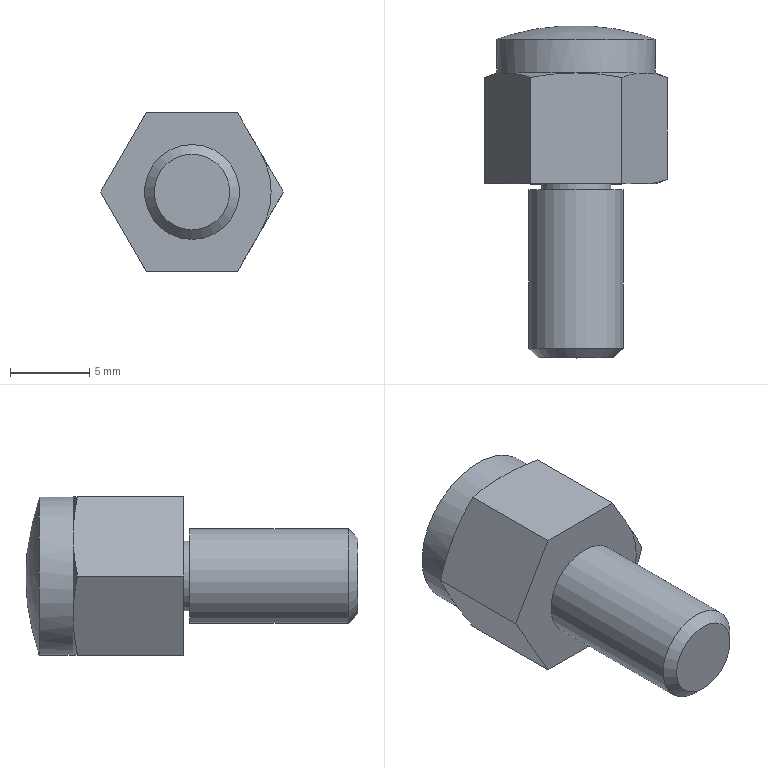Part | NX | features BREP 1 | 1 solid | 21 faces | box 11.547 x 21 x 10 mm | volume 1111 mm3 | plane 9 | cone 8 | cylinder 3 | sphere 1 | commonest cylinder face diameters 4.4 x1 6 x1 10 x1
STEP:
#1=CARTESIAN_POINT('',(4.33,0.5,-2.5));
#2=VERTEX_POINT('',#1);
#3=CARTESIAN_POINT('',(4.33,0.5,2.5));
#4=VERTEX_POINT('',#3);
#5=CARTESIAN_POINT('',(0.,0.5,0.));
#6=DIRECTION('',(0.,-1.,0.));
#7=DIRECTION('',(0.,0.,-1.));
#8=AXIS2_PLACEMENT_3D('',#5,#6,#7);
#9=CIRCLE('',#8,5.);
#10=EDGE_CURVE('',#2,#4,#9,.T.);
#11=ORIENTED_EDGE('',*,*,#10,.F.);
#12=CARTESIAN_POINT('',(5.774,0.7815,0.));
#13=VERTEX_POINT('',#12);
#14=CARTESIAN_POINT('',(4.33,0.5,-2.5));
#15=CARTESIAN_POINT('',(4.816,0.5,-1.659));
#16=CARTESIAN_POINT('',(5.296,0.6078,-0.8266));
#17=CARTESIAN_POINT('',(5.774,0.7815,0.));
#18=B_SPLINE_CURVE_WITH_KNOTS('',3,(#14,#15,#16,#17),.UNSPECIFIED.,.F.,.F.,(4,4),(0.,0.0029),.UNSPECIFIED.);
#19=EDGE_CURVE('',#2,#13,#18,.T.);
#20=ORIENTED_EDGE('',*,*,#19,.T.);
#21=CARTESIAN_POINT('',(5.774,0.7815,0.));
#22=CARTESIAN_POINT('',(5.296,0.6078,0.8266));
#23=CARTESIAN_POINT('',(4.816,0.5,1.659));
#24=CARTESIAN_POINT('',(4.33,0.5,2.5));
#25=B_SPLINE_CURVE_WITH_KNOTS('',3,(#21,#22,#23,#24),.UNSPECIFIED.,.F.,.F.,(4,4),(0.,0.0029),.UNSPECIFIED.);
#26=EDGE_CURVE('',#13,#4,#25,.T.);
#27=ORIENTED_EDGE('',*,*,#26,.T.);
#28=EDGE_LOOP('',(#11,#20,#27));
#29=FACE_BOUND('',#28,.T.);
#30=CARTESIAN_POINT('',(0.,4.,0.));
#31=DIRECTION('',(0.,1.,0.));
#32=DIRECTION('',(0.,0.,-1.));
#33=AXIS2_PLACEMENT_3D('',#30,#31,#32);
#34=CONICAL_SURFACE('',#33,14.616,1.222);
#35=ADVANCED_FACE('',(#29),#34,.T.);
#36=CARTESIAN_POINT('',(0.,0.5,-2.2));
#37=VERTEX_POINT('',#36);
#38=CARTESIAN_POINT('',(0.,0.5,0.));
#39=DIRECTION('',(0.,-1.,0.));
#40=DIRECTION('',(0.,0.,-1.));
#41=AXIS2_PLACEMENT_3D('',#38,#39,#40);
#42=CIRCLE('',#41,2.2);
#43=EDGE_CURVE('',#37,#37,#42,.T.);
#44=ORIENTED_EDGE('',*,*,#43,.F.);
#45=EDGE_LOOP('',(#44));
#46=FACE_BOUND('',#45,.T.);
#47=CARTESIAN_POINT('',(2.887,0.5,-5.));
#48=VERTEX_POINT('',#47);
#49=CARTESIAN_POINT('',(-2.887,0.5,-5.));
#50=VERTEX_POINT('',#49);
#51=CARTESIAN_POINT('',(5.,0.5,-5.));
#52=DIRECTION('',(-1.,0.,0.));
#53=VECTOR('',#52,1000.);
#54=LINE('',#51,#53);
#55=EDGE_CURVE('',#48,#50,#54,.T.);
#56=ORIENTED_EDGE('',*,*,#55,.F.);
#57=CARTESIAN_POINT('',(5.58,0.5,-0.3349));
#58=DIRECTION('',(-0.5,0.,-0.866));
#59=VECTOR('',#58,1000.);
#60=LINE('',#57,#59);
#61=EDGE_CURVE('',#2,#48,#60,.T.);
#62=ORIENTED_EDGE('',*,*,#61,.F.);
#63=ORIENTED_EDGE('',*,*,#10,.T.);
#64=CARTESIAN_POINT('',(2.887,0.5,5.));
#65=VERTEX_POINT('',#64);
#66=CARTESIAN_POINT('',(2.887,0.5,5.));
#67=DIRECTION('',(-0.5,0.,0.866));
#68=VECTOR('',#67,1000.);
#69=LINE('',#66,#68);
#70=EDGE_CURVE('',#4,#65,#69,.T.);
#71=ORIENTED_EDGE('',*,*,#70,.T.);
#72=CARTESIAN_POINT('',(-2.887,0.5,5.));
#73=VERTEX_POINT('',#72);
#74=CARTESIAN_POINT('',(-2.887,0.5,5.));
#75=DIRECTION('',(-1.,0.,0.));
#76=VECTOR('',#75,1000.);
#77=LINE('',#74,#76);
#78=EDGE_CURVE('',#65,#73,#77,.T.);
#79=ORIENTED_EDGE('',*,*,#78,.T.);
#80=CARTESIAN_POINT('',(-5.774,0.5,0.));
#81=VERTEX_POINT('',#80);
#82=CARTESIAN_POINT('',(-5.774,0.5,0.));
#83=DIRECTION('',(-0.5,0.,-0.866));
#84=VECTOR('',#83,1000.);
#85=LINE('',#82,#84);
#86=EDGE_CURVE('',#73,#81,#85,.T.);
#87=ORIENTED_EDGE('',*,*,#86,.T.);
#88=CARTESIAN_POINT('',(-3.08,0.5,-4.665));
#89=DIRECTION('',(-0.5,0.,0.866));
#90=VECTOR('',#89,1000.);
#91=LINE('',#88,#90);
#92=EDGE_CURVE('',#50,#81,#91,.T.);
#93=ORIENTED_EDGE('',*,*,#92,.F.);
#94=EDGE_LOOP('',(#56,#62,#63,#71,#79,#87,#93));
#95=FACE_BOUND('',#94,.T.);
#96=CARTESIAN_POINT('',(5.,0.5,0.));
#97=DIRECTION('',(0.,1.,0.));
#98=DIRECTION('',(0.,0.,-1.));
#99=AXIS2_PLACEMENT_3D('',#96,#97,#98);
#100=PLANE('',#99);
#101=ADVANCED_FACE('',(#46,#95),#100,.F.);
#102=CARTESIAN_POINT('',(-2.887,7.218,-5.));
#103=VERTEX_POINT('',#102);
#104=CARTESIAN_POINT('',(-2.887,15.,-5.));
#105=DIRECTION('',(0.,-1.,0.));
#106=VECTOR('',#105,1000.);
#107=LINE('',#104,#106);
#108=EDGE_CURVE('',#103,#50,#107,.T.);
#109=ORIENTED_EDGE('',*,*,#108,.T.);
#110=ORIENTED_EDGE('',*,*,#92,.T.);
#111=CARTESIAN_POINT('',(-5.774,7.218,0.));
#112=VERTEX_POINT('',#111);
#113=CARTESIAN_POINT('',(-5.774,15.,0.));
#114=DIRECTION('',(0.,-1.,0.));
#115=VECTOR('',#114,1000.);
#116=LINE('',#113,#115);
#117=EDGE_CURVE('',#112,#81,#116,.T.);
#118=ORIENTED_EDGE('',*,*,#117,.F.);
#119=CARTESIAN_POINT('',(-4.33,7.5,-2.5));
#120=VERTEX_POINT('',#119);
#121=CARTESIAN_POINT('',(-4.33,7.5,-2.5));
#122=CARTESIAN_POINT('',(-4.816,7.5,-1.659));
#123=CARTESIAN_POINT('',(-5.296,7.392,-0.8266));
#124=CARTESIAN_POINT('',(-5.774,7.218,0.));
#125=B_SPLINE_CURVE_WITH_KNOTS('',3,(#121,#122,#123,#124),.UNSPECIFIED.,.F.,.F.,(4,4),(0.,0.0029),.UNSPECIFIED.);
#126=EDGE_CURVE('',#120,#112,#125,.T.);
#127=ORIENTED_EDGE('',*,*,#126,.F.);
#128=CARTESIAN_POINT('',(-2.887,7.218,-5.));
#129=CARTESIAN_POINT('',(-3.364,7.392,-4.173));
#130=CARTESIAN_POINT('',(-3.844,7.5,-3.341));
#131=CARTESIAN_POINT('',(-4.33,7.5,-2.5));
#132=B_SPLINE_CURVE_WITH_KNOTS('',3,(#128,#129,#130,#131),.UNSPECIFIED.,.F.,.F.,(4,4),(0.,0.0029),.UNSPECIFIED.);
#133=EDGE_CURVE('',#103,#120,#132,.T.);
#134=ORIENTED_EDGE('',*,*,#133,.F.);
#135=EDGE_LOOP('',(#109,#110,#118,#127,#134));
#136=FACE_BOUND('',#135,.T.);
#137=CARTESIAN_POINT('',(-2.887,15.,-5.));
#138=DIRECTION('',(0.866,0.,0.5));
#139=DIRECTION('',(-0.5,0.,0.866));
#140=AXIS2_PLACEMENT_3D('',#137,#138,#139);
#141=PLANE('',#140);
#142=ADVANCED_FACE('',(#136),#141,.F.);
#143=CARTESIAN_POINT('',(2.887,7.218,-5.));
#144=VERTEX_POINT('',#143);
#145=CARTESIAN_POINT('',(2.887,15.,-5.));
#146=DIRECTION('',(0.,-1.,0.));
#147=VECTOR('',#146,1000.);
#148=LINE('',#145,#147);
#149=EDGE_CURVE('',#144,#48,#148,.T.);
#150=ORIENTED_EDGE('',*,*,#149,.T.);
#151=ORIENTED_EDGE('',*,*,#55,.T.);
#152=ORIENTED_EDGE('',*,*,#108,.F.);
#153=CARTESIAN_POINT('',(0.,7.5,-5.));
#154=VERTEX_POINT('',#153);
#155=CARTESIAN_POINT('',(0.,7.5,-5.));
#156=CARTESIAN_POINT('',(-0.9714,7.5,-5.));
#157=CARTESIAN_POINT('',(-1.932,7.392,-5.));
#158=CARTESIAN_POINT('',(-2.887,7.218,-5.));
#159=B_SPLINE_CURVE_WITH_KNOTS('',3,(#155,#156,#157,#158),.UNSPECIFIED.,.F.,.F.,(4,4),(0.,0.0029),.UNSPECIFIED.);
#160=EDGE_CURVE('',#154,#103,#159,.T.);
#161=ORIENTED_EDGE('',*,*,#160,.F.);
#162=CARTESIAN_POINT('',(2.887,7.218,-5.));
#163=CARTESIAN_POINT('',(1.932,7.392,-5.));
#164=CARTESIAN_POINT('',(0.9714,7.5,-5.));
#165=CARTESIAN_POINT('',(0.,7.5,-5.));
#166=B_SPLINE_CURVE_WITH_KNOTS('',3,(#162,#163,#164,#165),.UNSPECIFIED.,.F.,.F.,(4,4),(0.,0.0029),.UNSPECIFIED.);
#167=EDGE_CURVE('',#144,#154,#166,.T.);
#168=ORIENTED_EDGE('',*,*,#167,.F.);
#169=EDGE_LOOP('',(#150,#151,#152,#161,#168));
#170=FACE_BOUND('',#169,.T.);
#171=CARTESIAN_POINT('',(2.887,15.,-5.));
#172=DIRECTION('',(0.,0.,1.));
#173=DIRECTION('',(-1.,0.,0.));
#174=AXIS2_PLACEMENT_3D('',#171,#172,#173);
#175=PLANE('',#174);
#176=ADVANCED_FACE('',(#170),#175,.F.);
#177=CARTESIAN_POINT('',(5.774,7.218,0.));
#178=VERTEX_POINT('',#177);
#179=CARTESIAN_POINT('',(5.774,15.,0.));
#180=DIRECTION('',(0.,-1.,0.));
#181=VECTOR('',#180,1000.);
#182=LINE('',#179,#181);
#183=EDGE_CURVE('',#178,#13,#182,.T.);
#184=ORIENTED_EDGE('',*,*,#183,.T.);
#185=ORIENTED_EDGE('',*,*,#19,.F.);
#186=ORIENTED_EDGE('',*,*,#61,.T.);
#187=ORIENTED_EDGE('',*,*,#149,.F.);
#188=CARTESIAN_POINT('',(4.33,7.5,-2.5));
#189=VERTEX_POINT('',#188);
#190=CARTESIAN_POINT('',(4.33,7.5,-2.5));
#191=CARTESIAN_POINT('',(3.844,7.5,-3.341));
#192=CARTESIAN_POINT('',(3.364,7.392,-4.173));
#193=CARTESIAN_POINT('',(2.887,7.218,-5.));
#194=B_SPLINE_CURVE_WITH_KNOTS('',3,(#190,#191,#192,#193),.UNSPECIFIED.,.F.,.F.,(4,4),(0.,0.0029),.UNSPECIFIED.);
#195=EDGE_CURVE('',#189,#144,#194,.T.);
#196=ORIENTED_EDGE('',*,*,#195,.F.);
#197=CARTESIAN_POINT('',(5.774,7.218,0.));
#198=CARTESIAN_POINT('',(5.296,7.392,-0.8266));
#199=CARTESIAN_POINT('',(4.816,7.5,-1.659));
#200=CARTESIAN_POINT('',(4.33,7.5,-2.5));
#201=B_SPLINE_CURVE_WITH_KNOTS('',3,(#197,#198,#199,#200),.UNSPECIFIED.,.F.,.F.,(4,4),(0.,0.0029),.UNSPECIFIED.);
#202=EDGE_CURVE('',#178,#189,#201,.T.);
#203=ORIENTED_EDGE('',*,*,#202,.F.);
#204=EDGE_LOOP('',(#184,#185,#186,#187,#196,#203));
#205=FACE_BOUND('',#204,.T.);
#206=CARTESIAN_POINT('',(5.774,15.,0.));
#207=DIRECTION('',(-0.866,0.,0.5));
#208=DIRECTION('',(-0.5,0.,-0.866));
#209=AXIS2_PLACEMENT_3D('',#206,#207,#208);
#210=PLANE('',#209);
#211=ADVANCED_FACE('',(#205),#210,.F.);
#212=CARTESIAN_POINT('',(2.887,7.218,5.));
#213=VERTEX_POINT('',#212);
#214=CARTESIAN_POINT('',(2.887,15.,5.));
#215=DIRECTION('',(0.,-1.,0.));
#216=VECTOR('',#215,1000.);
#217=LINE('',#214,#216);
#218=EDGE_CURVE('',#213,#65,#217,.T.);
#219=ORIENTED_EDGE('',*,*,#218,.T.);
#220=ORIENTED_EDGE('',*,*,#70,.F.);
#221=ORIENTED_EDGE('',*,*,#26,.F.);
#222=ORIENTED_EDGE('',*,*,#183,.F.);
#223=CARTESIAN_POINT('',(4.33,7.5,2.5));
#224=VERTEX_POINT('',#223);
#225=CARTESIAN_POINT('',(4.33,7.5,2.5));
#226=CARTESIAN_POINT('',(4.816,7.5,1.659));
#227=CARTESIAN_POINT('',(5.296,7.392,0.8266));
#228=CARTESIAN_POINT('',(5.774,7.218,0.));
#229=B_SPLINE_CURVE_WITH_KNOTS('',3,(#225,#226,#227,#228),.UNSPECIFIED.,.F.,.F.,(4,4),(0.,0.0029),.UNSPECIFIED.);
#230=EDGE_CURVE('',#224,#178,#229,.T.);
#231=ORIENTED_EDGE('',*,*,#230,.F.);
#232=CARTESIAN_POINT('',(2.887,7.218,5.));
#233=CARTESIAN_POINT('',(3.364,7.392,4.173));
#234=CARTESIAN_POINT('',(3.844,7.5,3.341));
#235=CARTESIAN_POINT('',(4.33,7.5,2.5));
#236=B_SPLINE_CURVE_WITH_KNOTS('',3,(#232,#233,#234,#235),.UNSPECIFIED.,.F.,.F.,(4,4),(0.,0.0029),.UNSPECIFIED.);
#237=EDGE_CURVE('',#213,#224,#236,.T.);
#238=ORIENTED_EDGE('',*,*,#237,.F.);
#239=EDGE_LOOP('',(#219,#220,#221,#222,#231,#238));
#240=FACE_BOUND('',#239,.T.);
#241=CARTESIAN_POINT('',(2.887,15.,5.));
#242=DIRECTION('',(-0.866,0.,-0.5));
#243=DIRECTION('',(0.5,0.,-0.866));
#244=AXIS2_PLACEMENT_3D('',#241,#242,#243);
#245=PLANE('',#244);
#246=ADVANCED_FACE('',(#240),#245,.F.);
#247=CARTESIAN_POINT('',(-2.887,7.218,5.));
#248=VERTEX_POINT('',#247);
#249=CARTESIAN_POINT('',(-2.887,15.,5.));
#250=DIRECTION('',(0.,-1.,0.));
#251=VECTOR('',#250,1000.);
#252=LINE('',#249,#251);
#253=EDGE_CURVE('',#248,#73,#252,.T.);
#254=ORIENTED_EDGE('',*,*,#253,.T.);
#255=ORIENTED_EDGE('',*,*,#78,.F.);
#256=ORIENTED_EDGE('',*,*,#218,.F.);
#257=CARTESIAN_POINT('',(0.,7.5,5.));
#258=VERTEX_POINT('',#257);
#259=CARTESIAN_POINT('',(0.,7.5,5.));
#260=CARTESIAN_POINT('',(0.9714,7.5,5.));
#261=CARTESIAN_POINT('',(1.932,7.392,5.));
#262=CARTESIAN_POINT('',(2.887,7.218,5.));
#263=B_SPLINE_CURVE_WITH_KNOTS('',3,(#259,#260,#261,#262),.UNSPECIFIED.,.F.,.F.,(4,4),(0.,0.0029),.UNSPECIFIED.);
#264=EDGE_CURVE('',#258,#213,#263,.T.);
#265=ORIENTED_EDGE('',*,*,#264,.F.);
#266=CARTESIAN_POINT('',(-2.887,7.218,5.));
#267=CARTESIAN_POINT('',(-1.932,7.392,5.));
#268=CARTESIAN_POINT('',(-0.9714,7.5,5.));
#269=CARTESIAN_POINT('',(0.,7.5,5.));
#270=B_SPLINE_CURVE_WITH_KNOTS('',3,(#266,#267,#268,#269),.UNSPECIFIED.,.F.,.F.,(4,4),(0.,0.0029),.UNSPECIFIED.);
#271=EDGE_CURVE('',#248,#258,#270,.T.);
#272=ORIENTED_EDGE('',*,*,#271,.F.);
#273=EDGE_LOOP('',(#254,#255,#256,#265,#272));
#274=FACE_BOUND('',#273,.T.);
#275=CARTESIAN_POINT('',(-2.887,15.,5.));
#276=DIRECTION('',(0.,0.,-1.));
#277=DIRECTION('',(1.,0.,0.));
#278=AXIS2_PLACEMENT_3D('',#275,#276,#277);
#279=PLANE('',#278);
#280=ADVANCED_FACE('',(#274),#279,.F.);
#281=ORIENTED_EDGE('',*,*,#117,.T.);
#282=ORIENTED_EDGE('',*,*,#86,.F.);
#283=ORIENTED_EDGE('',*,*,#253,.F.);
#284=CARTESIAN_POINT('',(-4.33,7.5,2.5));
#285=VERTEX_POINT('',#284);
#286=CARTESIAN_POINT('',(-4.33,7.5,2.5));
#287=CARTESIAN_POINT('',(-3.844,7.5,3.341));
#288=CARTESIAN_POINT('',(-3.364,7.392,4.173));
#289=CARTESIAN_POINT('',(-2.887,7.218,5.));
#290=B_SPLINE_CURVE_WITH_KNOTS('',3,(#286,#287,#288,#289),.UNSPECIFIED.,.F.,.F.,(4,4),(0.,0.0029),.UNSPECIFIED.);
#291=EDGE_CURVE('',#285,#248,#290,.T.);
#292=ORIENTED_EDGE('',*,*,#291,.F.);
#293=CARTESIAN_POINT('',(-5.774,7.218,0.));
#294=CARTESIAN_POINT('',(-5.296,7.392,0.8266));
#295=CARTESIAN_POINT('',(-4.816,7.5,1.659));
#296=CARTESIAN_POINT('',(-4.33,7.5,2.5));
#297=B_SPLINE_CURVE_WITH_KNOTS('',3,(#293,#294,#295,#296),.UNSPECIFIED.,.F.,.F.,(4,4),(0.,0.0029),.UNSPECIFIED.);
#298=EDGE_CURVE('',#112,#285,#297,.T.);
#299=ORIENTED_EDGE('',*,*,#298,.F.);
#300=EDGE_LOOP('',(#281,#282,#283,#292,#299));
#301=FACE_BOUND('',#300,.T.);
#302=CARTESIAN_POINT('',(-5.774,15.,0.));
#303=DIRECTION('',(0.866,0.,-0.5));
#304=DIRECTION('',(0.5,0.,0.866));
#305=AXIS2_PLACEMENT_3D('',#302,#303,#304);
#306=PLANE('',#305);
#307=ADVANCED_FACE('',(#301),#306,.F.);
#308=CARTESIAN_POINT('',(0.,9.642,-5.));
#309=VERTEX_POINT('',#308);
#310=CARTESIAN_POINT('',(0.,9.642,0.));
#311=DIRECTION('',(0.,-1.,0.));
#312=DIRECTION('',(0.,0.,-1.));
#313=AXIS2_PLACEMENT_3D('',#310,#311,#312);
#314=CIRCLE('',#313,5.);
#315=EDGE_CURVE('',#309,#309,#314,.T.);
#316=ORIENTED_EDGE('',*,*,#315,.F.);
#317=EDGE_LOOP('',(#316));
#318=FACE_BOUND('',#317,.T.);
#319=CARTESIAN_POINT('',(0.,-4.5,0.));
#320=DIRECTION('',(0.,0.,1.));
#321=DIRECTION('',(-1.,0.,0.));
#322=AXIS2_PLACEMENT_3D('',#319,#320,#321);
#323=SPHERICAL_SURFACE('',#322,15.);
#324=ADVANCED_FACE('',(#318),#323,.T.);
#325=CARTESIAN_POINT('',(0.,7.5,0.));
#326=DIRECTION('',(0.,-1.,0.));
#327=DIRECTION('',(0.,0.,-1.));
#328=AXIS2_PLACEMENT_3D('',#325,#326,#327);
#329=CIRCLE('',#328,5.);
#330=EDGE_CURVE('',#154,#189,#329,.T.);
#331=ORIENTED_EDGE('',*,*,#330,.T.);
#332=ORIENTED_EDGE('',*,*,#195,.T.);
#333=ORIENTED_EDGE('',*,*,#167,.T.);
#334=EDGE_LOOP('',(#331,#332,#333));
#335=FACE_BOUND('',#334,.T.);
#336=CARTESIAN_POINT('',(0.,7.5,0.));
#337=DIRECTION('',(0.,-1.,0.));
#338=DIRECTION('',(0.,0.,1.));
#339=AXIS2_PLACEMENT_3D('',#336,#337,#338);
#340=CONICAL_SURFACE('',#339,5.,1.222);
#341=ADVANCED_FACE('',(#335),#340,.T.);
#342=ORIENTED_EDGE('',*,*,#291,.T.);
#343=ORIENTED_EDGE('',*,*,#271,.T.);
#344=CARTESIAN_POINT('',(0.,7.5,0.));
#345=DIRECTION('',(0.,-1.,0.));
#346=DIRECTION('',(0.,0.,-1.));
#347=AXIS2_PLACEMENT_3D('',#344,#345,#346);
#348=CIRCLE('',#347,5.);
#349=EDGE_CURVE('',#258,#285,#348,.T.);
#350=ORIENTED_EDGE('',*,*,#349,.T.);
#351=EDGE_LOOP('',(#342,#343,#350));
#352=FACE_BOUND('',#351,.T.);
#353=CARTESIAN_POINT('',(0.,7.5,0.));
#354=DIRECTION('',(0.,-1.,0.));
#355=DIRECTION('',(0.,0.,1.));
#356=AXIS2_PLACEMENT_3D('',#353,#354,#355);
#357=CONICAL_SURFACE('',#356,5.,1.222);
#358=ADVANCED_FACE('',(#352),#357,.T.);
#359=CARTESIAN_POINT('',(0.,7.5,0.));
#360=DIRECTION('',(0.,-1.,0.));
#361=DIRECTION('',(0.,0.,-1.));
#362=AXIS2_PLACEMENT_3D('',#359,#360,#361);
#363=CIRCLE('',#362,5.);
#364=EDGE_CURVE('',#285,#120,#363,.T.);
#365=ORIENTED_EDGE('',*,*,#364,.T.);
#366=ORIENTED_EDGE('',*,*,#126,.T.);
#367=ORIENTED_EDGE('',*,*,#298,.T.);
#368=EDGE_LOOP('',(#365,#366,#367));
#369=FACE_BOUND('',#368,.T.);
#370=CARTESIAN_POINT('',(0.,7.5,0.));
#371=DIRECTION('',(0.,-1.,0.));
#372=DIRECTION('',(0.,0.,1.));
#373=AXIS2_PLACEMENT_3D('',#370,#371,#372);
#374=CONICAL_SURFACE('',#373,5.,1.222);
#375=ADVANCED_FACE('',(#369),#374,.T.);
#376=ORIENTED_EDGE('',*,*,#264,.T.);
#377=ORIENTED_EDGE('',*,*,#237,.T.);
#378=CARTESIAN_POINT('',(0.,7.5,0.));
#379=DIRECTION('',(0.,-1.,0.));
#380=DIRECTION('',(0.,0.,-1.));
#381=AXIS2_PLACEMENT_3D('',#378,#379,#380);
#382=CIRCLE('',#381,5.);
#383=EDGE_CURVE('',#224,#258,#382,.T.);
#384=ORIENTED_EDGE('',*,*,#383,.T.);
#385=EDGE_LOOP('',(#376,#377,#384));
#386=FACE_BOUND('',#385,.T.);
#387=CARTESIAN_POINT('',(0.,7.5,0.));
#388=DIRECTION('',(0.,-1.,0.));
#389=DIRECTION('',(0.,0.,1.));
#390=AXIS2_PLACEMENT_3D('',#387,#388,#389);
#391=CONICAL_SURFACE('',#390,5.,1.222);
#392=ADVANCED_FACE('',(#386),#391,.T.);
#393=CARTESIAN_POINT('',(0.,7.5,0.));
#394=DIRECTION('',(0.,-1.,0.));
#395=DIRECTION('',(0.,0.,-1.));
#396=AXIS2_PLACEMENT_3D('',#393,#394,#395);
#397=CIRCLE('',#396,5.);
#398=EDGE_CURVE('',#189,#224,#397,.T.);
#399=ORIENTED_EDGE('',*,*,#398,.F.);
#400=ORIENTED_EDGE('',*,*,#330,.F.);
#401=CARTESIAN_POINT('',(0.,7.5,0.));
#402=DIRECTION('',(0.,-1.,0.));
#403=DIRECTION('',(0.,0.,-1.));
#404=AXIS2_PLACEMENT_3D('',#401,#402,#403);
#405=CIRCLE('',#404,5.);
#406=EDGE_CURVE('',#120,#154,#405,.T.);
#407=ORIENTED_EDGE('',*,*,#406,.F.);
#408=ORIENTED_EDGE('',*,*,#364,.F.);
#409=ORIENTED_EDGE('',*,*,#349,.F.);
#410=ORIENTED_EDGE('',*,*,#383,.F.);
#411=EDGE_LOOP('',(#399,#400,#407,#408,#409,#410));
#412=FACE_BOUND('',#411,.T.);
#413=ORIENTED_EDGE('',*,*,#315,.T.);
#414=EDGE_LOOP('',(#413));
#415=FACE_BOUND('',#414,.T.);
#416=CARTESIAN_POINT('',(0.,-10.5,0.));
#417=DIRECTION('',(0.,-1.,0.));
#418=DIRECTION('',(0.,0.,1.));
#419=AXIS2_PLACEMENT_3D('',#416,#417,#418);
#420=CYLINDRICAL_SURFACE('',#419,5.);
#421=ADVANCED_FACE('',(#412,#415),#420,.T.);
#422=ORIENTED_EDGE('',*,*,#398,.T.);
#423=ORIENTED_EDGE('',*,*,#230,.T.);
#424=ORIENTED_EDGE('',*,*,#202,.T.);
#425=EDGE_LOOP('',(#422,#423,#424));
#426=FACE_BOUND('',#425,.T.);
#427=CARTESIAN_POINT('',(0.,7.5,0.));
#428=DIRECTION('',(0.,-1.,0.));
#429=DIRECTION('',(0.,0.,1.));
#430=AXIS2_PLACEMENT_3D('',#427,#428,#429);
#431=CONICAL_SURFACE('',#430,5.,1.222);
#432=ADVANCED_FACE('',(#426),#431,.T.);
#433=ORIENTED_EDGE('',*,*,#406,.T.);
#434=ORIENTED_EDGE('',*,*,#160,.T.);
#435=ORIENTED_EDGE('',*,*,#133,.T.);
#436=EDGE_LOOP('',(#433,#434,#435));
#437=FACE_BOUND('',#436,.T.);
#438=CARTESIAN_POINT('',(0.,7.5,0.));
#439=DIRECTION('',(0.,-1.,0.));
#440=DIRECTION('',(0.,0.,1.));
#441=AXIS2_PLACEMENT_3D('',#438,#439,#440);
#442=CONICAL_SURFACE('',#441,5.,1.222);
#443=ADVANCED_FACE('',(#437),#442,.T.);
#444=ORIENTED_EDGE('',*,*,#43,.T.);
#445=EDGE_LOOP('',(#444));
#446=FACE_BOUND('',#445,.T.);
#447=CARTESIAN_POINT('',(0.,0.1333,-2.2));
#448=VERTEX_POINT('',#447);
#449=CARTESIAN_POINT('',(0.,0.1333,0.));
#450=DIRECTION('',(0.,-1.,0.));
#451=DIRECTION('',(0.,0.,-1.));
#452=AXIS2_PLACEMENT_3D('',#449,#450,#451);
#453=CIRCLE('',#452,2.2);
#454=EDGE_CURVE('',#448,#448,#453,.T.);
#455=ORIENTED_EDGE('',*,*,#454,.F.);
#456=EDGE_LOOP('',(#455));
#457=FACE_BOUND('',#456,.T.);
#458=CARTESIAN_POINT('',(0.,0.5,0.));
#459=DIRECTION('',(0.,-1.,0.));
#460=DIRECTION('',(0.,0.,1.));
#461=AXIS2_PLACEMENT_3D('',#458,#459,#460);
#462=CYLINDRICAL_SURFACE('',#461,2.2);
#463=ADVANCED_FACE('',(#446,#457),#462,.T.);
#464=CARTESIAN_POINT('',(0.,-10.5,-2.386));
#465=VERTEX_POINT('',#464);
#466=CARTESIAN_POINT('',(0.,-10.5,0.));
#467=DIRECTION('',(0.,-1.,0.));
#468=DIRECTION('',(0.,0.,-1.));
#469=AXIS2_PLACEMENT_3D('',#466,#467,#468);
#470=CIRCLE('',#469,2.386);
#471=EDGE_CURVE('',#465,#465,#470,.T.);
#472=ORIENTED_EDGE('',*,*,#471,.T.);
#473=EDGE_LOOP('',(#472));
#474=FACE_BOUND('',#473,.T.);
#475=CARTESIAN_POINT('',(0.,-10.5,0.));
#476=DIRECTION('',(0.,-1.,0.));
#477=DIRECTION('',(0.,0.,1.));
#478=AXIS2_PLACEMENT_3D('',#475,#476,#477);
#479=PLANE('',#478);
#480=ADVANCED_FACE('',(#474),#479,.T.);
#481=CARTESIAN_POINT('',(0.,-9.886,-3.));
#482=VERTEX_POINT('',#481);
#483=CARTESIAN_POINT('',(0.,-9.886,0.));
#484=DIRECTION('',(0.,1.,0.));
#485=DIRECTION('',(0.,0.,-1.));
#486=AXIS2_PLACEMENT_3D('',#483,#484,#485);
#487=CIRCLE('',#486,3.);
#488=EDGE_CURVE('',#482,#482,#487,.T.);
#489=ORIENTED_EDGE('',*,*,#488,.T.);
#490=EDGE_LOOP('',(#489));
#491=FACE_BOUND('',#490,.T.);
#492=CARTESIAN_POINT('',(0.,0.1333,-3.));
#493=VERTEX_POINT('',#492);
#494=CARTESIAN_POINT('',(0.,0.1333,0.));
#495=DIRECTION('',(0.,-1.,0.));
#496=DIRECTION('',(0.,0.,-1.));
#497=AXIS2_PLACEMENT_3D('',#494,#495,#496);
#498=CIRCLE('',#497,3.);
#499=EDGE_CURVE('',#493,#493,#498,.T.);
#500=ORIENTED_EDGE('',*,*,#499,.T.);
#501=EDGE_LOOP('',(#500));
#502=FACE_BOUND('',#501,.T.);
#503=CARTESIAN_POINT('',(0.,0.5,0.));
#504=DIRECTION('',(0.,-1.,0.));
#505=DIRECTION('',(0.,0.,1.));
#506=AXIS2_PLACEMENT_3D('',#503,#504,#505);
#507=CYLINDRICAL_SURFACE('',#506,3.);
#508=ADVANCED_FACE('',(#491,#502),#507,.T.);
#509=ORIENTED_EDGE('',*,*,#454,.T.);
#510=EDGE_LOOP('',(#509));
#511=FACE_BOUND('',#510,.T.);
#512=ORIENTED_EDGE('',*,*,#499,.F.);
#513=EDGE_LOOP('',(#512));
#514=FACE_BOUND('',#513,.T.);
#515=CARTESIAN_POINT('',(3.,0.1333,0.));
#516=DIRECTION('',(0.,1.,0.));
#517=DIRECTION('',(0.,0.,-1.));
#518=AXIS2_PLACEMENT_3D('',#515,#516,#517);
#519=PLANE('',#518);
#520=ADVANCED_FACE('',(#511,#514),#519,.T.);
#521=ORIENTED_EDGE('',*,*,#488,.F.);
#522=EDGE_LOOP('',(#521));
#523=FACE_BOUND('',#522,.T.);
#524=ORIENTED_EDGE('',*,*,#471,.F.);
#525=EDGE_LOOP('',(#524));
#526=FACE_BOUND('',#525,.T.);
#527=CARTESIAN_POINT('',(0.,-10.5,0.));
#528=DIRECTION('',(0.,1.,0.));
#529=DIRECTION('',(0.,0.,-1.));
#530=AXIS2_PLACEMENT_3D('',#527,#528,#529);
#531=CONICAL_SURFACE('',#530,2.386,0.7854);
#532=ADVANCED_FACE('',(#523,#526),#531,.T.);
#533=CLOSED_SHELL('',(#35,#101,#142,#176,#211,#246,#280,#307,#324,#341,#358,#375,#392,#421,#432,#443,#463,#480,#508,#520,#532));
#534=MANIFOLD_SOLID_BREP('',#533);
#535=(LENGTH_UNIT()NAMED_UNIT(*)SI_UNIT(.MILLI.,.METRE.));
#536=UNCERTAINTY_MEASURE_WITH_UNIT(LENGTH_MEASURE(0.0508),#535,'','');
#537=(NAMED_UNIT(*)PLANE_ANGLE_UNIT()SI_UNIT($,.RADIAN.));
#538=(NAMED_UNIT(*)SI_UNIT($,.STERADIAN.)SOLID_ANGLE_UNIT());
#539=(GEOMETRIC_REPRESENTATION_CONTEXT(3)GLOBAL_UNCERTAINTY_ASSIGNED_CONTEXT((#536))GLOBAL_UNIT_ASSIGNED_CONTEXT((#535,#537,#538))REPRESENTATION_CONTEXT('',''));
#540=ADVANCED_BREP_SHAPE_REPRESENTATION('',(#534),#539);